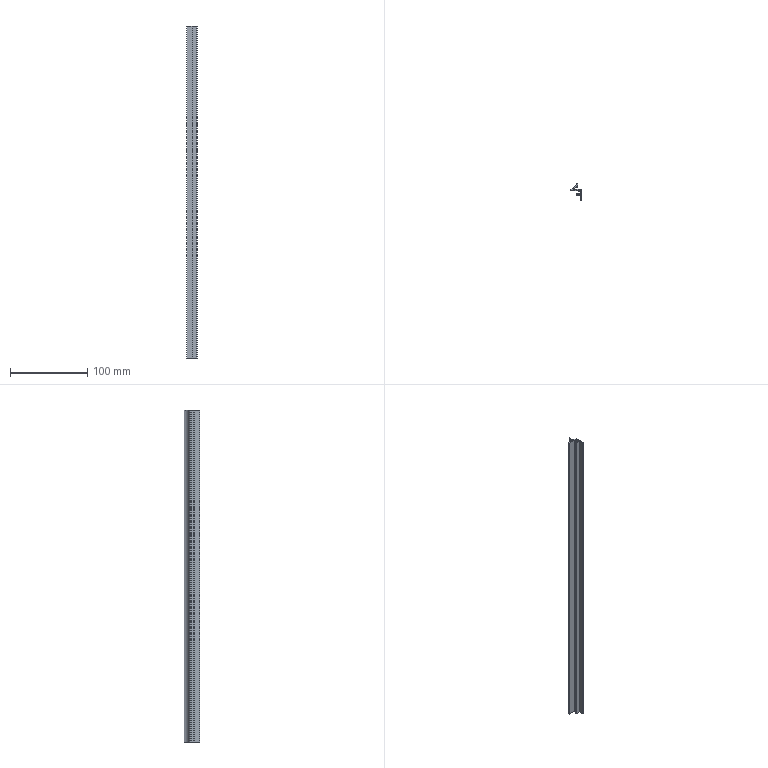Part | SolidWorks | features BaseBody 1, ICE 1, MoveFace 1 | 1 solid | 27 faces | box 14 x 20.3 x 430 mm | volume 21894 mm3 | plane 20 | cylinder 7 | commonest cylinder face diameters 0.387 x2 0.8 x2 0.4 x1 20 x1 22 x1
STEP:
#1=CARTESIAN_POINT('',(-5.304,-0.625,200.));
#2=VERTEX_POINT('',#1);
#3=CARTESIAN_POINT('',(-5.449,-0.8125,200.));
#4=VERTEX_POINT('',#3);
#5=CARTESIAN_POINT('',(-5.255,-0.8125,200.));
#6=DIRECTION('',(0.,0.,1.));
#7=DIRECTION('',(-1.,0.,0.));
#8=AXIS2_PLACEMENT_3D('',#5,#6,#7);
#9=CIRCLE('',#8,0.1937);
#10=EDGE_CURVE('',#2,#4,#9,.T.);
#11=ORIENTED_EDGE('',*,*,#10,.T.);
#12=CARTESIAN_POINT('',(-5.449,-0.8125,-230.));
#13=VERTEX_POINT('',#12);
#14=CARTESIAN_POINT('',(-5.449,-0.8125,230.));
#15=DIRECTION('',(0.,0.,-1.));
#16=VECTOR('',#15,1000.);
#17=LINE('',#14,#16);
#18=EDGE_CURVE('',#4,#13,#17,.T.);
#19=ORIENTED_EDGE('',*,*,#18,.T.);
#20=CARTESIAN_POINT('',(-5.304,-0.625,-230.));
#21=VERTEX_POINT('',#20);
#22=CARTESIAN_POINT('',(-5.255,-0.8125,-230.));
#23=DIRECTION('',(0.,0.,-1.));
#24=DIRECTION('',(1.,0.,0.));
#25=AXIS2_PLACEMENT_3D('',#22,#23,#24);
#26=CIRCLE('',#25,0.1937);
#27=EDGE_CURVE('',#13,#21,#26,.T.);
#28=ORIENTED_EDGE('',*,*,#27,.T.);
#29=CARTESIAN_POINT('',(-5.304,-0.625,230.));
#30=DIRECTION('',(0.,0.,-1.));
#31=VECTOR('',#30,1000.);
#32=LINE('',#29,#31);
#33=EDGE_CURVE('',#2,#21,#32,.T.);
#34=ORIENTED_EDGE('',*,*,#33,.F.);
#35=EDGE_LOOP('',(#11,#19,#28,#34));
#36=FACE_OUTER_BOUND('',#35,.T.);
#37=CARTESIAN_POINT('',(-5.255,-0.8125,230.));
#38=DIRECTION('',(0.,0.,-1.));
#39=DIRECTION('',(-1.,0.,0.));
#40=AXIS2_PLACEMENT_3D('',#37,#38,#39);
#41=CYLINDRICAL_SURFACE('',#40,0.1937);
#42=ADVANCED_FACE('',(#36),#41,.F.);
#43=CARTESIAN_POINT('',(5.,-1.,-230.));
#44=VERTEX_POINT('',#43);
#45=CARTESIAN_POINT('',(5.,-14.3,-230.));
#46=VERTEX_POINT('',#45);
#47=CARTESIAN_POINT('',(5.,29.623,-230.));
#48=DIRECTION('',(0.,-1.,0.));
#49=VECTOR('',#48,1000.);
#50=LINE('',#47,#49);
#51=EDGE_CURVE('',#44,#46,#50,.T.);
#52=ORIENTED_EDGE('',*,*,#51,.F.);
#53=CARTESIAN_POINT('',(5.,-1.,200.));
#54=VERTEX_POINT('',#53);
#55=CARTESIAN_POINT('',(5.,-1.,230.));
#56=DIRECTION('',(0.,0.,-1.));
#57=VECTOR('',#56,1000.);
#58=LINE('',#55,#57);
#59=EDGE_CURVE('',#54,#44,#58,.T.);
#60=ORIENTED_EDGE('',*,*,#59,.F.);
#61=CARTESIAN_POINT('',(5.,-14.3,200.));
#62=VERTEX_POINT('',#61);
#63=CARTESIAN_POINT('',(5.,-14.3,200.));
#64=DIRECTION('',(0.,1.,0.));
#65=VECTOR('',#64,1000.);
#66=LINE('',#63,#65);
#67=EDGE_CURVE('',#62,#54,#66,.T.);
#68=ORIENTED_EDGE('',*,*,#67,.F.);
#69=CARTESIAN_POINT('',(5.,-14.3,230.));
#70=DIRECTION('',(0.,0.,1.));
#71=VECTOR('',#70,1000.);
#72=LINE('',#69,#71);
#73=EDGE_CURVE('',#46,#62,#72,.T.);
#74=ORIENTED_EDGE('',*,*,#73,.F.);
#75=EDGE_LOOP('',(#52,#60,#68,#74));
#76=FACE_OUTER_BOUND('',#75,.T.);
#77=CARTESIAN_POINT('',(5.,-14.3,230.));
#78=DIRECTION('',(-1.,0.,0.));
#79=DIRECTION('',(0.,0.,1.));
#80=AXIS2_PLACEMENT_3D('',#77,#78,#79);
#81=PLANE('',#80);
#82=ADVANCED_FACE('',(#76),#81,.F.);
#83=CARTESIAN_POINT('',(-9.,-2.,-230.));
#84=VERTEX_POINT('',#83);
#85=CARTESIAN_POINT('',(-9.,-2.,200.));
#86=VERTEX_POINT('',#85);
#87=CARTESIAN_POINT('',(-9.,-2.,230.));
#88=DIRECTION('',(0.,0.,1.));
#89=VECTOR('',#88,1000.);
#90=LINE('',#87,#89);
#91=EDGE_CURVE('',#84,#86,#90,.T.);
#92=ORIENTED_EDGE('',*,*,#91,.F.);
#93=CARTESIAN_POINT('',(0.9,-2.,-230.));
#94=VERTEX_POINT('',#93);
#95=CARTESIAN_POINT('',(5.,-2.,-230.));
#96=DIRECTION('',(-1.,0.,0.));
#97=VECTOR('',#96,1000.);
#98=LINE('',#95,#97);
#99=EDGE_CURVE('',#94,#84,#98,.T.);
#100=ORIENTED_EDGE('',*,*,#99,.F.);
#101=CARTESIAN_POINT('',(0.9,-2.,200.));
#102=VERTEX_POINT('',#101);
#103=CARTESIAN_POINT('',(0.9,-2.,230.));
#104=DIRECTION('',(0.,0.,-1.));
#105=VECTOR('',#104,1000.);
#106=LINE('',#103,#105);
#107=EDGE_CURVE('',#102,#94,#106,.T.);
#108=ORIENTED_EDGE('',*,*,#107,.F.);
#109=CARTESIAN_POINT('',(5.,-2.,200.));
#110=DIRECTION('',(1.,0.,0.));
#111=VECTOR('',#110,1000.);
#112=LINE('',#109,#111);
#113=EDGE_CURVE('',#86,#102,#112,.T.);
#114=ORIENTED_EDGE('',*,*,#113,.F.);
#115=EDGE_LOOP('',(#92,#100,#108,#114));
#116=FACE_OUTER_BOUND('',#115,.T.);
#117=CARTESIAN_POINT('',(-9.,-2.,230.));
#118=DIRECTION('',(0.,1.,0.));
#119=DIRECTION('',(0.,0.,1.));
#120=AXIS2_PLACEMENT_3D('',#117,#118,#119);
#121=PLANE('',#120);
#122=ADVANCED_FACE('',(#116),#121,.F.);
#123=CARTESIAN_POINT('',(4.,-6.,200.));
#124=VERTEX_POINT('',#123);
#125=CARTESIAN_POINT('',(4.,-3.,200.));
#126=VERTEX_POINT('',#125);
#127=CARTESIAN_POINT('',(4.,29.623,200.));
#128=DIRECTION('',(0.,1.,0.));
#129=VECTOR('',#128,1000.);
#130=LINE('',#127,#129);
#131=EDGE_CURVE('',#124,#126,#130,.T.);
#132=ORIENTED_EDGE('',*,*,#131,.F.);
#133=CARTESIAN_POINT('',(1.,-6.,200.));
#134=VERTEX_POINT('',#133);
#135=CARTESIAN_POINT('',(5.,-6.,200.));
#136=DIRECTION('',(1.,0.,0.));
#137=VECTOR('',#136,1000.);
#138=LINE('',#135,#137);
#139=EDGE_CURVE('',#134,#124,#138,.T.);
#140=ORIENTED_EDGE('',*,*,#139,.F.);
#141=CARTESIAN_POINT('',(1.,-6.7,200.));
#142=VERTEX_POINT('',#141);
#143=CARTESIAN_POINT('',(1.,-6.,200.));
#144=DIRECTION('',(0.,-1.,0.));
#145=VECTOR('',#144,1000.);
#146=LINE('',#143,#145);
#147=EDGE_CURVE('',#134,#142,#146,.T.);
#148=ORIENTED_EDGE('',*,*,#147,.T.);
#149=CARTESIAN_POINT('',(-1.7,-6.7,200.));
#150=VERTEX_POINT('',#149);
#151=CARTESIAN_POINT('',(5.,-6.7,200.));
#152=DIRECTION('',(1.,0.,0.));
#153=VECTOR('',#152,1000.);
#154=LINE('',#151,#153);
#155=EDGE_CURVE('',#150,#142,#154,.T.);
#156=ORIENTED_EDGE('',*,*,#155,.F.);
#157=CARTESIAN_POINT('',(-1.7,-7.7,200.));
#158=VERTEX_POINT('',#157);
#159=CARTESIAN_POINT('',(-1.7,-6.7,200.));
#160=DIRECTION('',(0.,-1.,0.));
#161=VECTOR('',#160,1000.);
#162=LINE('',#159,#161);
#163=EDGE_CURVE('',#150,#158,#162,.T.);
#164=ORIENTED_EDGE('',*,*,#163,.T.);
#165=CARTESIAN_POINT('',(4.,-7.7,200.));
#166=VERTEX_POINT('',#165);
#167=CARTESIAN_POINT('',(5.,-7.7,200.));
#168=DIRECTION('',(-1.,0.,0.));
#169=VECTOR('',#168,1000.);
#170=LINE('',#167,#169);
#171=EDGE_CURVE('',#166,#158,#170,.T.);
#172=ORIENTED_EDGE('',*,*,#171,.F.);
#173=CARTESIAN_POINT('',(4.,-14.3,200.));
#174=VERTEX_POINT('',#173);
#175=CARTESIAN_POINT('',(4.,29.623,200.));
#176=DIRECTION('',(0.,1.,0.));
#177=VECTOR('',#176,1000.);
#178=LINE('',#175,#177);
#179=EDGE_CURVE('',#174,#166,#178,.T.);
#180=ORIENTED_EDGE('',*,*,#179,.F.);
#181=CARTESIAN_POINT('',(5.,-14.3,200.));
#182=DIRECTION('',(-1.,0.,0.));
#183=VECTOR('',#182,1000.);
#184=LINE('',#181,#183);
#185=EDGE_CURVE('',#62,#174,#184,.T.);
#186=ORIENTED_EDGE('',*,*,#185,.F.);
#187=ORIENTED_EDGE('',*,*,#67,.T.);
#188=CARTESIAN_POINT('',(-5.207,-1.,200.));
#189=VERTEX_POINT('',#188);
#190=CARTESIAN_POINT('',(5.,-1.,200.));
#191=DIRECTION('',(1.,0.,0.));
#192=VECTOR('',#191,1000.);
#193=LINE('',#190,#192);
#194=EDGE_CURVE('',#189,#54,#193,.T.);
#195=ORIENTED_EDGE('',*,*,#194,.F.);
#196=CARTESIAN_POINT('',(-5.255,-0.8125,200.));
#197=DIRECTION('',(0.,0.,1.));
#198=DIRECTION('',(-1.,0.,0.));
#199=AXIS2_PLACEMENT_3D('',#196,#197,#198);
#200=CIRCLE('',#199,0.1937);
#201=EDGE_CURVE('',#4,#189,#200,.T.);
#202=ORIENTED_EDGE('',*,*,#201,.F.);
#203=ORIENTED_EDGE('',*,*,#10,.F.);
#204=CARTESIAN_POINT('',(-1.368,3.063,200.));
#205=VERTEX_POINT('',#204);
#206=CARTESIAN_POINT('',(-10.628,9.,200.));
#207=DIRECTION('',(0.,0.,1.));
#208=DIRECTION('',(-1.,0.,0.));
#209=AXIS2_PLACEMENT_3D('',#206,#207,#208);
#210=CIRCLE('',#209,11.);
#211=EDGE_CURVE('',#2,#205,#210,.T.);
#212=ORIENTED_EDGE('',*,*,#211,.T.);
#213=CARTESIAN_POINT('',(-1.,2.955,200.));
#214=VERTEX_POINT('',#213);
#215=CARTESIAN_POINT('',(-1.2,2.955,200.));
#216=DIRECTION('',(0.,0.,1.));
#217=DIRECTION('',(-1.,0.,0.));
#218=AXIS2_PLACEMENT_3D('',#215,#216,#217);
#219=CIRCLE('',#218,0.2);
#220=EDGE_CURVE('',#214,#205,#219,.T.);
#221=ORIENTED_EDGE('',*,*,#220,.F.);
#222=CARTESIAN_POINT('',(-1.,1.5,200.));
#223=VERTEX_POINT('',#222);
#224=CARTESIAN_POINT('',(-1.,2.955,200.));
#225=DIRECTION('',(0.,1.,0.));
#226=VECTOR('',#225,1000.);
#227=LINE('',#224,#226);
#228=EDGE_CURVE('',#223,#214,#227,.T.);
#229=ORIENTED_EDGE('',*,*,#228,.F.);
#230=CARTESIAN_POINT('',(0.,1.5,200.));
#231=VERTEX_POINT('',#230);
#232=CARTESIAN_POINT('',(-1.,1.5,200.));
#233=DIRECTION('',(-1.,0.,0.));
#234=VECTOR('',#233,1000.);
#235=LINE('',#232,#234);
#236=EDGE_CURVE('',#231,#223,#235,.T.);
#237=ORIENTED_EDGE('',*,*,#236,.F.);
#238=CARTESIAN_POINT('',(0.,6.,200.));
#239=VERTEX_POINT('',#238);
#240=CARTESIAN_POINT('',(0.,1.5,200.));
#241=DIRECTION('',(0.,-1.,0.));
#242=VECTOR('',#241,1000.);
#243=LINE('',#240,#242);
#244=EDGE_CURVE('',#239,#231,#243,.T.);
#245=ORIENTED_EDGE('',*,*,#244,.F.);
#246=CARTESIAN_POINT('',(-0.8,6.,200.));
#247=VERTEX_POINT('',#246);
#248=CARTESIAN_POINT('',(0.,6.,200.));
#249=DIRECTION('',(1.,0.,0.));
#250=VECTOR('',#249,1000.);
#251=LINE('',#248,#250);
#252=EDGE_CURVE('',#247,#239,#251,.T.);
#253=ORIENTED_EDGE('',*,*,#252,.F.);
#254=CARTESIAN_POINT('',(-1.178,5.731,200.));
#255=VERTEX_POINT('',#254);
#256=CARTESIAN_POINT('',(-0.8,5.6,200.));
#257=DIRECTION('',(0.,0.,1.));
#258=DIRECTION('',(-1.,0.,0.));
#259=AXIS2_PLACEMENT_3D('',#256,#257,#258);
#260=CIRCLE('',#259,0.4);
#261=EDGE_CURVE('',#247,#255,#260,.T.);
#262=ORIENTED_EDGE('',*,*,#261,.T.);
#263=CARTESIAN_POINT('',(-8.678,-0.8077,200.));
#264=VERTEX_POINT('',#263);
#265=CARTESIAN_POINT('',(-10.628,9.,200.));
#266=DIRECTION('',(0.,0.,1.));
#267=DIRECTION('',(-1.,0.,0.));
#268=AXIS2_PLACEMENT_3D('',#265,#266,#267);
#269=CIRCLE('',#268,10.);
#270=EDGE_CURVE('',#264,#255,#269,.T.);
#271=ORIENTED_EDGE('',*,*,#270,.F.);
#272=CARTESIAN_POINT('',(-9.,-1.2,200.));
#273=VERTEX_POINT('',#272);
#274=CARTESIAN_POINT('',(-8.6,-1.2,200.));
#275=DIRECTION('',(0.,0.,1.));
#276=DIRECTION('',(-1.,0.,0.));
#277=AXIS2_PLACEMENT_3D('',#274,#275,#276);
#278=CIRCLE('',#277,0.4);
#279=EDGE_CURVE('',#264,#273,#278,.T.);
#280=ORIENTED_EDGE('',*,*,#279,.T.);
#281=CARTESIAN_POINT('',(-9.,8.,200.));
#282=DIRECTION('',(0.,-1.,0.));
#283=VECTOR('',#282,1000.);
#284=LINE('',#281,#283);
#285=EDGE_CURVE('',#273,#86,#284,.T.);
#286=ORIENTED_EDGE('',*,*,#285,.T.);
#287=ORIENTED_EDGE('',*,*,#113,.T.);
#288=CARTESIAN_POINT('',(0.9,-3.,200.));
#289=VERTEX_POINT('',#288);
#290=CARTESIAN_POINT('',(0.9,29.623,200.));
#291=DIRECTION('',(0.,1.,0.));
#292=VECTOR('',#291,1000.);
#293=LINE('',#290,#292);
#294=EDGE_CURVE('',#289,#102,#293,.T.);
#295=ORIENTED_EDGE('',*,*,#294,.F.);
#296=CARTESIAN_POINT('',(5.,-3.,200.));
#297=DIRECTION('',(-1.,0.,0.));
#298=VECTOR('',#297,1000.);
#299=LINE('',#296,#298);
#300=EDGE_CURVE('',#126,#289,#299,.T.);
#301=ORIENTED_EDGE('',*,*,#300,.F.);
#302=EDGE_LOOP('',(#132,#140,#148,#156,#164,#172,#180,#186,#187,#195,#202,#203,#212,#221,#229,#237,#245,#253,#262,#271,#280,#286,#287,#295,#301));
#303=FACE_OUTER_BOUND('',#302,.T.);
#304=CARTESIAN_POINT('',(5.,29.623,200.));
#305=DIRECTION('',(0.,0.,-1.));
#306=DIRECTION('',(-1.,0.,0.));
#307=AXIS2_PLACEMENT_3D('',#304,#305,#306);
#308=PLANE('',#307);
#309=ADVANCED_FACE('',(#303),#308,.F.);
#310=ORIENTED_EDGE('',*,*,#185,.T.);
#311=CARTESIAN_POINT('',(4.,-14.3,-230.));
#312=VERTEX_POINT('',#311);
#313=CARTESIAN_POINT('',(4.,-14.3,230.));
#314=DIRECTION('',(0.,0.,1.));
#315=VECTOR('',#314,1000.);
#316=LINE('',#313,#315);
#317=EDGE_CURVE('',#312,#174,#316,.T.);
#318=ORIENTED_EDGE('',*,*,#317,.F.);
#319=CARTESIAN_POINT('',(5.,-14.3,-230.));
#320=DIRECTION('',(-1.,0.,0.));
#321=VECTOR('',#320,1000.);
#322=LINE('',#319,#321);
#323=EDGE_CURVE('',#46,#312,#322,.T.);
#324=ORIENTED_EDGE('',*,*,#323,.F.);
#325=ORIENTED_EDGE('',*,*,#73,.T.);
#326=EDGE_LOOP('',(#310,#318,#324,#325));
#327=FACE_OUTER_BOUND('',#326,.T.);
#328=CARTESIAN_POINT('',(4.,-14.3,230.));
#329=DIRECTION('',(0.,1.,0.));
#330=DIRECTION('',(0.,0.,1.));
#331=AXIS2_PLACEMENT_3D('',#328,#329,#330);
#332=PLANE('',#331);
#333=ADVANCED_FACE('',(#327),#332,.F.);
#334=ORIENTED_EDGE('',*,*,#51,.T.);
#335=ORIENTED_EDGE('',*,*,#323,.T.);
#336=CARTESIAN_POINT('',(4.,-7.7,-230.));
#337=VERTEX_POINT('',#336);
#338=CARTESIAN_POINT('',(4.,-7.7,-230.));
#339=DIRECTION('',(0.,-1.,0.));
#340=VECTOR('',#339,1000.);
#341=LINE('',#338,#340);
#342=EDGE_CURVE('',#337,#312,#341,.T.);
#343=ORIENTED_EDGE('',*,*,#342,.F.);
#344=CARTESIAN_POINT('',(-1.7,-7.7,-230.));
#345=VERTEX_POINT('',#344);
#346=CARTESIAN_POINT('',(-1.7,-7.7,-230.));
#347=DIRECTION('',(1.,0.,0.));
#348=VECTOR('',#347,1000.);
#349=LINE('',#346,#348);
#350=EDGE_CURVE('',#345,#337,#349,.T.);
#351=ORIENTED_EDGE('',*,*,#350,.F.);
#352=CARTESIAN_POINT('',(-1.7,-6.7,-230.));
#353=VERTEX_POINT('',#352);
#354=CARTESIAN_POINT('',(-1.7,29.623,-230.));
#355=DIRECTION('',(0.,1.,0.));
#356=VECTOR('',#355,1000.);
#357=LINE('',#354,#356);
#358=EDGE_CURVE('',#345,#353,#357,.T.);
#359=ORIENTED_EDGE('',*,*,#358,.T.);
#360=CARTESIAN_POINT('',(1.,-6.7,-230.));
#361=VERTEX_POINT('',#360);
#362=CARTESIAN_POINT('',(1.,-6.7,-230.));
#363=DIRECTION('',(-1.,0.,0.));
#364=VECTOR('',#363,1000.);
#365=LINE('',#362,#364);
#366=EDGE_CURVE('',#361,#353,#365,.T.);
#367=ORIENTED_EDGE('',*,*,#366,.F.);
#368=CARTESIAN_POINT('',(1.,-6.,-230.));
#369=VERTEX_POINT('',#368);
#370=CARTESIAN_POINT('',(1.,29.623,-230.));
#371=DIRECTION('',(0.,1.,0.));
#372=VECTOR('',#371,1000.);
#373=LINE('',#370,#372);
#374=EDGE_CURVE('',#361,#369,#373,.T.);
#375=ORIENTED_EDGE('',*,*,#374,.T.);
#376=CARTESIAN_POINT('',(4.,-6.,-230.));
#377=VERTEX_POINT('',#376);
#378=CARTESIAN_POINT('',(4.,-6.,-230.));
#379=DIRECTION('',(-1.,0.,0.));
#380=VECTOR('',#379,1000.);
#381=LINE('',#378,#380);
#382=EDGE_CURVE('',#377,#369,#381,.T.);
#383=ORIENTED_EDGE('',*,*,#382,.F.);
#384=CARTESIAN_POINT('',(4.,-3.,-230.));
#385=VERTEX_POINT('',#384);
#386=CARTESIAN_POINT('',(4.,-3.,-230.));
#387=DIRECTION('',(0.,-1.,0.));
#388=VECTOR('',#387,1000.);
#389=LINE('',#386,#388);
#390=EDGE_CURVE('',#385,#377,#389,.T.);
#391=ORIENTED_EDGE('',*,*,#390,.F.);
#392=CARTESIAN_POINT('',(0.9,-3.,-230.));
#393=VERTEX_POINT('',#392);
#394=CARTESIAN_POINT('',(0.9,-3.,-230.));
#395=DIRECTION('',(1.,0.,0.));
#396=VECTOR('',#395,1000.);
#397=LINE('',#394,#396);
#398=EDGE_CURVE('',#393,#385,#397,.T.);
#399=ORIENTED_EDGE('',*,*,#398,.F.);
#400=CARTESIAN_POINT('',(0.9,-2.,-230.));
#401=DIRECTION('',(0.,-1.,0.));
#402=VECTOR('',#401,1000.);
#403=LINE('',#400,#402);
#404=EDGE_CURVE('',#94,#393,#403,.T.);
#405=ORIENTED_EDGE('',*,*,#404,.F.);
#406=ORIENTED_EDGE('',*,*,#99,.T.);
#407=CARTESIAN_POINT('',(-9.,-1.2,-230.));
#408=VERTEX_POINT('',#407);
#409=CARTESIAN_POINT('',(-9.,-1.2,-230.));
#410=DIRECTION('',(0.,-1.,0.));
#411=VECTOR('',#410,1000.);
#412=LINE('',#409,#411);
#413=EDGE_CURVE('',#408,#84,#412,.T.);
#414=ORIENTED_EDGE('',*,*,#413,.F.);
#415=CARTESIAN_POINT('',(-8.678,-0.8077,-230.));
#416=VERTEX_POINT('',#415);
#417=CARTESIAN_POINT('',(-8.6,-1.2,-230.));
#418=DIRECTION('',(0.,0.,-1.));
#419=DIRECTION('',(1.,0.,0.));
#420=AXIS2_PLACEMENT_3D('',#417,#418,#419);
#421=CIRCLE('',#420,0.4);
#422=EDGE_CURVE('',#408,#416,#421,.T.);
#423=ORIENTED_EDGE('',*,*,#422,.T.);
#424=CARTESIAN_POINT('',(-1.178,5.731,-230.));
#425=VERTEX_POINT('',#424);
#426=CARTESIAN_POINT('',(-10.628,9.,-230.));
#427=DIRECTION('',(0.,0.,-1.));
#428=DIRECTION('',(1.,0.,0.));
#429=AXIS2_PLACEMENT_3D('',#426,#427,#428);
#430=CIRCLE('',#429,10.);
#431=EDGE_CURVE('',#425,#416,#430,.T.);
#432=ORIENTED_EDGE('',*,*,#431,.F.);
#433=CARTESIAN_POINT('',(-0.8,6.,-230.));
#434=VERTEX_POINT('',#433);
#435=CARTESIAN_POINT('',(-0.8,5.6,-230.));
#436=DIRECTION('',(0.,0.,-1.));
#437=DIRECTION('',(1.,0.,0.));
#438=AXIS2_PLACEMENT_3D('',#435,#436,#437);
#439=CIRCLE('',#438,0.4);
#440=EDGE_CURVE('',#425,#434,#439,.T.);
#441=ORIENTED_EDGE('',*,*,#440,.T.);
#442=CARTESIAN_POINT('',(0.,6.,-230.));
#443=VERTEX_POINT('',#442);
#444=CARTESIAN_POINT('',(0.,6.,-230.));
#445=DIRECTION('',(-1.,0.,0.));
#446=VECTOR('',#445,1000.);
#447=LINE('',#444,#446);
#448=EDGE_CURVE('',#443,#434,#447,.T.);
#449=ORIENTED_EDGE('',*,*,#448,.F.);
#450=CARTESIAN_POINT('',(0.,1.5,-230.));
#451=VERTEX_POINT('',#450);
#452=CARTESIAN_POINT('',(0.,1.5,-230.));
#453=DIRECTION('',(0.,1.,0.));
#454=VECTOR('',#453,1000.);
#455=LINE('',#452,#454);
#456=EDGE_CURVE('',#451,#443,#455,.T.);
#457=ORIENTED_EDGE('',*,*,#456,.F.);
#458=CARTESIAN_POINT('',(-1.,1.5,-230.));
#459=VERTEX_POINT('',#458);
#460=CARTESIAN_POINT('',(-1.,1.5,-230.));
#461=DIRECTION('',(1.,0.,0.));
#462=VECTOR('',#461,1000.);
#463=LINE('',#460,#462);
#464=EDGE_CURVE('',#459,#451,#463,.T.);
#465=ORIENTED_EDGE('',*,*,#464,.F.);
#466=CARTESIAN_POINT('',(-1.,2.955,-230.));
#467=VERTEX_POINT('',#466);
#468=CARTESIAN_POINT('',(-1.,2.955,-230.));
#469=DIRECTION('',(0.,-1.,0.));
#470=VECTOR('',#469,1000.);
#471=LINE('',#468,#470);
#472=EDGE_CURVE('',#467,#459,#471,.T.);
#473=ORIENTED_EDGE('',*,*,#472,.F.);
#474=CARTESIAN_POINT('',(-1.368,3.063,-230.));
#475=VERTEX_POINT('',#474);
#476=CARTESIAN_POINT('',(-1.2,2.955,-230.));
#477=DIRECTION('',(0.,0.,-1.));
#478=DIRECTION('',(1.,0.,0.));
#479=AXIS2_PLACEMENT_3D('',#476,#477,#478);
#480=CIRCLE('',#479,0.2);
#481=EDGE_CURVE('',#475,#467,#480,.T.);
#482=ORIENTED_EDGE('',*,*,#481,.F.);
#483=CARTESIAN_POINT('',(-10.628,9.,-230.));
#484=DIRECTION('',(0.,0.,-1.));
#485=DIRECTION('',(1.,0.,0.));
#486=AXIS2_PLACEMENT_3D('',#483,#484,#485);
#487=CIRCLE('',#486,11.);
#488=EDGE_CURVE('',#475,#21,#487,.T.);
#489=ORIENTED_EDGE('',*,*,#488,.T.);
#490=ORIENTED_EDGE('',*,*,#27,.F.);
#491=CARTESIAN_POINT('',(-5.207,-1.,-230.));
#492=VERTEX_POINT('',#491);
#493=CARTESIAN_POINT('',(-5.255,-0.8125,-230.));
#494=DIRECTION('',(0.,0.,-1.));
#495=DIRECTION('',(1.,0.,0.));
#496=AXIS2_PLACEMENT_3D('',#493,#494,#495);
#497=CIRCLE('',#496,0.1937);
#498=EDGE_CURVE('',#492,#13,#497,.T.);
#499=ORIENTED_EDGE('',*,*,#498,.F.);
#500=CARTESIAN_POINT('',(5.,-1.,-230.));
#501=DIRECTION('',(-1.,0.,0.));
#502=VECTOR('',#501,1000.);
#503=LINE('',#500,#502);
#504=EDGE_CURVE('',#44,#492,#503,.T.);
#505=ORIENTED_EDGE('',*,*,#504,.F.);
#506=EDGE_LOOP('',(#334,#335,#343,#351,#359,#367,#375,#383,#391,#399,#405,#406,#414,#423,#432,#441,#449,#457,#465,#473,#482,#489,#490,#499,#505));
#507=FACE_OUTER_BOUND('',#506,.T.);
#508=CARTESIAN_POINT('',(5.,29.623,-230.));
#509=DIRECTION('',(0.,0.,1.));
#510=DIRECTION('',(1.,0.,0.));
#511=AXIS2_PLACEMENT_3D('',#508,#509,#510);
#512=PLANE('',#511);
#513=ADVANCED_FACE('',(#507),#512,.F.);
#514=ORIENTED_EDGE('',*,*,#59,.T.);
#515=ORIENTED_EDGE('',*,*,#504,.T.);
#516=CARTESIAN_POINT('',(-5.207,-1.,230.));
#517=DIRECTION('',(0.,0.,-1.));
#518=VECTOR('',#517,1000.);
#519=LINE('',#516,#518);
#520=EDGE_CURVE('',#189,#492,#519,.T.);
#521=ORIENTED_EDGE('',*,*,#520,.F.);
#522=ORIENTED_EDGE('',*,*,#194,.T.);
#523=EDGE_LOOP('',(#514,#515,#521,#522));
#524=FACE_OUTER_BOUND('',#523,.T.);
#525=CARTESIAN_POINT('',(5.,-1.,230.));
#526=DIRECTION('',(0.,-1.,0.));
#527=DIRECTION('',(0.,0.,-1.));
#528=AXIS2_PLACEMENT_3D('',#525,#526,#527);
#529=PLANE('',#528);
#530=ADVANCED_FACE('',(#524),#529,.F.);
#531=CARTESIAN_POINT('',(-9.,-1.2,230.));
#532=DIRECTION('',(0.,0.,1.));
#533=VECTOR('',#532,1000.);
#534=LINE('',#531,#533);
#535=EDGE_CURVE('',#408,#273,#534,.T.);
#536=ORIENTED_EDGE('',*,*,#535,.F.);
#537=ORIENTED_EDGE('',*,*,#413,.T.);
#538=ORIENTED_EDGE('',*,*,#91,.T.);
#539=ORIENTED_EDGE('',*,*,#285,.F.);
#540=EDGE_LOOP('',(#536,#537,#538,#539));
#541=FACE_OUTER_BOUND('',#540,.T.);
#542=CARTESIAN_POINT('',(-9.,-1.2,230.));
#543=DIRECTION('',(1.,0.,0.));
#544=DIRECTION('',(0.,0.,-1.));
#545=AXIS2_PLACEMENT_3D('',#542,#543,#544);
#546=PLANE('',#545);
#547=ADVANCED_FACE('',(#541),#546,.F.);
#548=ORIENTED_EDGE('',*,*,#294,.T.);
#549=ORIENTED_EDGE('',*,*,#107,.T.);
#550=ORIENTED_EDGE('',*,*,#404,.T.);
#551=CARTESIAN_POINT('',(0.9,-3.,230.));
#552=DIRECTION('',(0.,0.,-1.));
#553=VECTOR('',#552,1000.);
#554=LINE('',#551,#553);
#555=EDGE_CURVE('',#289,#393,#554,.T.);
#556=ORIENTED_EDGE('',*,*,#555,.F.);
#557=EDGE_LOOP('',(#548,#549,#550,#556));
#558=FACE_OUTER_BOUND('',#557,.T.);
#559=CARTESIAN_POINT('',(0.9,-2.,230.));
#560=DIRECTION('',(1.,0.,0.));
#561=DIRECTION('',(0.,0.,-1.));
#562=AXIS2_PLACEMENT_3D('',#559,#560,#561);
#563=PLANE('',#562);
#564=ADVANCED_FACE('',(#558),#563,.F.);
#565=ORIENTED_EDGE('',*,*,#300,.T.);
#566=ORIENTED_EDGE('',*,*,#555,.T.);
#567=ORIENTED_EDGE('',*,*,#398,.T.);
#568=CARTESIAN_POINT('',(4.,-3.,230.));
#569=DIRECTION('',(0.,0.,-1.));
#570=VECTOR('',#569,1000.);
#571=LINE('',#568,#570);
#572=EDGE_CURVE('',#126,#385,#571,.T.);
#573=ORIENTED_EDGE('',*,*,#572,.F.);
#574=EDGE_LOOP('',(#565,#566,#567,#573));
#575=FACE_OUTER_BOUND('',#574,.T.);
#576=CARTESIAN_POINT('',(0.9,-3.,230.));
#577=DIRECTION('',(0.,1.,0.));
#578=DIRECTION('',(0.,0.,1.));
#579=AXIS2_PLACEMENT_3D('',#576,#577,#578);
#580=PLANE('',#579);
#581=ADVANCED_FACE('',(#575),#580,.F.);
#582=ORIENTED_EDGE('',*,*,#131,.T.);
#583=ORIENTED_EDGE('',*,*,#572,.T.);
#584=ORIENTED_EDGE('',*,*,#390,.T.);
#585=CARTESIAN_POINT('',(4.,-6.,230.));
#586=DIRECTION('',(0.,0.,-1.));
#587=VECTOR('',#586,1000.);
#588=LINE('',#585,#587);
#589=EDGE_CURVE('',#124,#377,#588,.T.);
#590=ORIENTED_EDGE('',*,*,#589,.F.);
#591=EDGE_LOOP('',(#582,#583,#584,#590));
#592=FACE_OUTER_BOUND('',#591,.T.);
#593=CARTESIAN_POINT('',(4.,-3.,230.));
#594=DIRECTION('',(1.,0.,0.));
#595=DIRECTION('',(0.,0.,-1.));
#596=AXIS2_PLACEMENT_3D('',#593,#594,#595);
#597=PLANE('',#596);
#598=ADVANCED_FACE('',(#592),#597,.F.);
#599=ORIENTED_EDGE('',*,*,#139,.T.);
#600=ORIENTED_EDGE('',*,*,#589,.T.);
#601=ORIENTED_EDGE('',*,*,#382,.T.);
#602=CARTESIAN_POINT('',(1.,-6.,230.));
#603=DIRECTION('',(0.,0.,-1.));
#604=VECTOR('',#603,1000.);
#605=LINE('',#602,#604);
#606=EDGE_CURVE('',#134,#369,#605,.T.);
#607=ORIENTED_EDGE('',*,*,#606,.F.);
#608=EDGE_LOOP('',(#599,#600,#601,#607));
#609=FACE_OUTER_BOUND('',#608,.T.);
#610=CARTESIAN_POINT('',(4.,-6.,230.));
#611=DIRECTION('',(0.,-1.,0.));
#612=DIRECTION('',(0.,0.,-1.));
#613=AXIS2_PLACEMENT_3D('',#610,#611,#612);
#614=PLANE('',#613);
#615=ADVANCED_FACE('',(#609),#614,.F.);
#616=ORIENTED_EDGE('',*,*,#155,.T.);
#617=CARTESIAN_POINT('',(1.,-6.7,230.));
#618=DIRECTION('',(0.,0.,1.));
#619=VECTOR('',#618,1000.);
#620=LINE('',#617,#619);
#621=EDGE_CURVE('',#361,#142,#620,.T.);
#622=ORIENTED_EDGE('',*,*,#621,.F.);
#623=ORIENTED_EDGE('',*,*,#366,.T.);
#624=CARTESIAN_POINT('',(-1.7,-6.7,230.));
#625=DIRECTION('',(0.,0.,-1.));
#626=VECTOR('',#625,1000.);
#627=LINE('',#624,#626);
#628=EDGE_CURVE('',#150,#353,#627,.T.);
#629=ORIENTED_EDGE('',*,*,#628,.F.);
#630=EDGE_LOOP('',(#616,#622,#623,#629));
#631=FACE_OUTER_BOUND('',#630,.T.);
#632=CARTESIAN_POINT('',(1.,-6.7,230.));
#633=DIRECTION('',(0.,-1.,0.));
#634=DIRECTION('',(0.,0.,-1.));
#635=AXIS2_PLACEMENT_3D('',#632,#633,#634);
#636=PLANE('',#635);
#637=ADVANCED_FACE('',(#631),#636,.F.);
#638=ORIENTED_EDGE('',*,*,#171,.T.);
#639=CARTESIAN_POINT('',(-1.7,-7.7,230.));
#640=DIRECTION('',(0.,0.,1.));
#641=VECTOR('',#640,1000.);
#642=LINE('',#639,#641);
#643=EDGE_CURVE('',#345,#158,#642,.T.);
#644=ORIENTED_EDGE('',*,*,#643,.F.);
#645=ORIENTED_EDGE('',*,*,#350,.T.);
#646=CARTESIAN_POINT('',(4.,-7.7,230.));
#647=DIRECTION('',(0.,0.,-1.));
#648=VECTOR('',#647,1000.);
#649=LINE('',#646,#648);
#650=EDGE_CURVE('',#166,#337,#649,.T.);
#651=ORIENTED_EDGE('',*,*,#650,.F.);
#652=EDGE_LOOP('',(#638,#644,#645,#651));
#653=FACE_OUTER_BOUND('',#652,.T.);
#654=CARTESIAN_POINT('',(-1.7,-7.7,230.));
#655=DIRECTION('',(0.,1.,0.));
#656=DIRECTION('',(0.,0.,1.));
#657=AXIS2_PLACEMENT_3D('',#654,#655,#656);
#658=PLANE('',#657);
#659=ADVANCED_FACE('',(#653),#658,.F.);
#660=ORIENTED_EDGE('',*,*,#179,.T.);
#661=ORIENTED_EDGE('',*,*,#650,.T.);
#662=ORIENTED_EDGE('',*,*,#342,.T.);
#663=ORIENTED_EDGE('',*,*,#317,.T.);
#664=EDGE_LOOP('',(#660,#661,#662,#663));
#665=FACE_OUTER_BOUND('',#664,.T.);
#666=CARTESIAN_POINT('',(4.,-7.7,230.));
#667=DIRECTION('',(1.,0.,0.));
#668=DIRECTION('',(0.,0.,-1.));
#669=AXIS2_PLACEMENT_3D('',#666,#667,#668);
#670=PLANE('',#669);
#671=ADVANCED_FACE('',(#665),#670,.F.);
#672=ORIENTED_EDGE('',*,*,#18,.F.);
#673=ORIENTED_EDGE('',*,*,#201,.T.);
#674=ORIENTED_EDGE('',*,*,#520,.T.);
#675=ORIENTED_EDGE('',*,*,#498,.T.);
#676=EDGE_LOOP('',(#672,#673,#674,#675));
#677=FACE_OUTER_BOUND('',#676,.T.);
#678=CARTESIAN_POINT('',(-5.255,-0.8125,230.));
#679=DIRECTION('',(0.,0.,-1.));
#680=DIRECTION('',(-1.,0.,0.));
#681=AXIS2_PLACEMENT_3D('',#678,#679,#680);
#682=CYLINDRICAL_SURFACE('',#681,0.1937);
#683=ADVANCED_FACE('',(#677),#682,.F.);
#684=CARTESIAN_POINT('',(-1.,2.955,230.));
#685=DIRECTION('',(0.,0.,1.));
#686=VECTOR('',#685,1000.);
#687=LINE('',#684,#686);
#688=EDGE_CURVE('',#467,#214,#687,.T.);
#689=ORIENTED_EDGE('',*,*,#688,.F.);
#690=ORIENTED_EDGE('',*,*,#472,.T.);
#691=CARTESIAN_POINT('',(-1.,1.5,230.));
#692=DIRECTION('',(0.,0.,-1.));
#693=VECTOR('',#692,1000.);
#694=LINE('',#691,#693);
#695=EDGE_CURVE('',#223,#459,#694,.T.);
#696=ORIENTED_EDGE('',*,*,#695,.F.);
#697=ORIENTED_EDGE('',*,*,#228,.T.);
#698=EDGE_LOOP('',(#689,#690,#696,#697));
#699=FACE_OUTER_BOUND('',#698,.T.);
#700=CARTESIAN_POINT('',(-1.,2.955,230.));
#701=DIRECTION('',(1.,0.,0.));
#702=DIRECTION('',(0.,0.,-1.));
#703=AXIS2_PLACEMENT_3D('',#700,#701,#702);
#704=PLANE('',#703);
#705=ADVANCED_FACE('',(#699),#704,.F.);
#706=ORIENTED_EDGE('',*,*,#488,.F.);
#707=CARTESIAN_POINT('',(-1.368,3.063,230.));
#708=DIRECTION('',(0.,0.,1.));
#709=VECTOR('',#708,1000.);
#710=LINE('',#707,#709);
#711=EDGE_CURVE('',#475,#205,#710,.T.);
#712=ORIENTED_EDGE('',*,*,#711,.T.);
#713=ORIENTED_EDGE('',*,*,#211,.F.);
#714=ORIENTED_EDGE('',*,*,#33,.T.);
#715=EDGE_LOOP('',(#706,#712,#713,#714));
#716=FACE_OUTER_BOUND('',#715,.T.);
#717=CARTESIAN_POINT('',(-10.628,9.,230.));
#718=DIRECTION('',(0.,0.,-1.));
#719=DIRECTION('',(-1.,0.,0.));
#720=AXIS2_PLACEMENT_3D('',#717,#718,#719);
#721=CYLINDRICAL_SURFACE('',#720,11.);
#722=ADVANCED_FACE('',(#716),#721,.T.);
#723=CARTESIAN_POINT('',(-1.178,5.731,230.));
#724=DIRECTION('',(0.,0.,1.));
#725=VECTOR('',#724,1000.);
#726=LINE('',#723,#725);
#727=EDGE_CURVE('',#425,#255,#726,.T.);
#728=ORIENTED_EDGE('',*,*,#727,.F.);
#729=ORIENTED_EDGE('',*,*,#431,.T.);
#730=CARTESIAN_POINT('',(-8.678,-0.8077,230.));
#731=DIRECTION('',(0.,0.,-1.));
#732=VECTOR('',#731,1000.);
#733=LINE('',#730,#732);
#734=EDGE_CURVE('',#264,#416,#733,.T.);
#735=ORIENTED_EDGE('',*,*,#734,.F.);
#736=ORIENTED_EDGE('',*,*,#270,.T.);
#737=EDGE_LOOP('',(#728,#729,#735,#736));
#738=FACE_OUTER_BOUND('',#737,.T.);
#739=CARTESIAN_POINT('',(-10.628,9.,230.));
#740=DIRECTION('',(0.,0.,-1.));
#741=DIRECTION('',(-1.,0.,0.));
#742=AXIS2_PLACEMENT_3D('',#739,#740,#741);
#743=CYLINDRICAL_SURFACE('',#742,10.);
#744=ADVANCED_FACE('',(#738),#743,.F.);
#745=CARTESIAN_POINT('',(0.,1.5,230.));
#746=DIRECTION('',(0.,0.,1.));
#747=VECTOR('',#746,1000.);
#748=LINE('',#745,#747);
#749=EDGE_CURVE('',#451,#231,#748,.T.);
#750=ORIENTED_EDGE('',*,*,#749,.F.);
#751=ORIENTED_EDGE('',*,*,#456,.T.);
#752=CARTESIAN_POINT('',(0.,6.,230.));
#753=DIRECTION('',(0.,0.,-1.));
#754=VECTOR('',#753,1000.);
#755=LINE('',#752,#754);
#756=EDGE_CURVE('',#239,#443,#755,.T.);
#757=ORIENTED_EDGE('',*,*,#756,.F.);
#758=ORIENTED_EDGE('',*,*,#244,.T.);
#759=EDGE_LOOP('',(#750,#751,#757,#758));
#760=FACE_OUTER_BOUND('',#759,.T.);
#761=CARTESIAN_POINT('',(0.,1.5,230.));
#762=DIRECTION('',(-1.,0.,0.));
#763=DIRECTION('',(0.,0.,1.));
#764=AXIS2_PLACEMENT_3D('',#761,#762,#763);
#765=PLANE('',#764);
#766=ADVANCED_FACE('',(#760),#765,.F.);
#767=ORIENTED_EDGE('',*,*,#422,.F.);
#768=ORIENTED_EDGE('',*,*,#535,.T.);
#769=ORIENTED_EDGE('',*,*,#279,.F.);
#770=ORIENTED_EDGE('',*,*,#734,.T.);
#771=EDGE_LOOP('',(#767,#768,#769,#770));
#772=FACE_OUTER_BOUND('',#771,.T.);
#773=CARTESIAN_POINT('',(-8.6,-1.2,230.));
#774=DIRECTION('',(0.,0.,-1.));
#775=DIRECTION('',(-1.,0.,0.));
#776=AXIS2_PLACEMENT_3D('',#773,#774,#775);
#777=CYLINDRICAL_SURFACE('',#776,0.4);
#778=ADVANCED_FACE('',(#772),#777,.T.);
#779=ORIENTED_EDGE('',*,*,#147,.F.);
#780=ORIENTED_EDGE('',*,*,#606,.T.);
#781=ORIENTED_EDGE('',*,*,#374,.F.);
#782=ORIENTED_EDGE('',*,*,#621,.T.);
#783=EDGE_LOOP('',(#779,#780,#781,#782));
#784=FACE_OUTER_BOUND('',#783,.T.);
#785=CARTESIAN_POINT('',(1.,-6.,230.));
#786=DIRECTION('',(1.,0.,0.));
#787=DIRECTION('',(0.,0.,-1.));
#788=AXIS2_PLACEMENT_3D('',#785,#786,#787);
#789=PLANE('',#788);
#790=ADVANCED_FACE('',(#784),#789,.F.);
#791=ORIENTED_EDGE('',*,*,#163,.F.);
#792=ORIENTED_EDGE('',*,*,#628,.T.);
#793=ORIENTED_EDGE('',*,*,#358,.F.);
#794=ORIENTED_EDGE('',*,*,#643,.T.);
#795=EDGE_LOOP('',(#791,#792,#793,#794));
#796=FACE_OUTER_BOUND('',#795,.T.);
#797=CARTESIAN_POINT('',(-1.7,-6.7,230.));
#798=DIRECTION('',(1.,0.,0.));
#799=DIRECTION('',(0.,0.,-1.));
#800=AXIS2_PLACEMENT_3D('',#797,#798,#799);
#801=PLANE('',#800);
#802=ADVANCED_FACE('',(#796),#801,.F.);
#803=ORIENTED_EDGE('',*,*,#711,.F.);
#804=ORIENTED_EDGE('',*,*,#481,.T.);
#805=ORIENTED_EDGE('',*,*,#688,.T.);
#806=ORIENTED_EDGE('',*,*,#220,.T.);
#807=EDGE_LOOP('',(#803,#804,#805,#806));
#808=FACE_OUTER_BOUND('',#807,.T.);
#809=CARTESIAN_POINT('',(-1.2,2.955,230.));
#810=DIRECTION('',(0.,0.,-1.));
#811=DIRECTION('',(-1.,0.,0.));
#812=AXIS2_PLACEMENT_3D('',#809,#810,#811);
#813=CYLINDRICAL_SURFACE('',#812,0.2);
#814=ADVANCED_FACE('',(#808),#813,.F.);
#815=ORIENTED_EDGE('',*,*,#695,.T.);
#816=ORIENTED_EDGE('',*,*,#464,.T.);
#817=ORIENTED_EDGE('',*,*,#749,.T.);
#818=ORIENTED_EDGE('',*,*,#236,.T.);
#819=EDGE_LOOP('',(#815,#816,#817,#818));
#820=FACE_OUTER_BOUND('',#819,.T.);
#821=CARTESIAN_POINT('',(-1.,1.5,230.));
#822=DIRECTION('',(0.,1.,0.));
#823=DIRECTION('',(0.,0.,1.));
#824=AXIS2_PLACEMENT_3D('',#821,#822,#823);
#825=PLANE('',#824);
#826=ADVANCED_FACE('',(#820),#825,.F.);
#827=ORIENTED_EDGE('',*,*,#440,.F.);
#828=ORIENTED_EDGE('',*,*,#727,.T.);
#829=ORIENTED_EDGE('',*,*,#261,.F.);
#830=CARTESIAN_POINT('',(-0.8,6.,230.));
#831=DIRECTION('',(0.,0.,-1.));
#832=VECTOR('',#831,1000.);
#833=LINE('',#830,#832);
#834=EDGE_CURVE('',#247,#434,#833,.T.);
#835=ORIENTED_EDGE('',*,*,#834,.T.);
#836=EDGE_LOOP('',(#827,#828,#829,#835));
#837=FACE_OUTER_BOUND('',#836,.T.);
#838=CARTESIAN_POINT('',(-0.8,5.6,230.));
#839=DIRECTION('',(0.,0.,-1.));
#840=DIRECTION('',(-1.,0.,0.));
#841=AXIS2_PLACEMENT_3D('',#838,#839,#840);
#842=CYLINDRICAL_SURFACE('',#841,0.4);
#843=ADVANCED_FACE('',(#837),#842,.T.);
#844=ORIENTED_EDGE('',*,*,#756,.T.);
#845=ORIENTED_EDGE('',*,*,#448,.T.);
#846=ORIENTED_EDGE('',*,*,#834,.F.);
#847=ORIENTED_EDGE('',*,*,#252,.T.);
#848=EDGE_LOOP('',(#844,#845,#846,#847));
#849=FACE_OUTER_BOUND('',#848,.T.);
#850=CARTESIAN_POINT('',(0.,6.,230.));
#851=DIRECTION('',(0.,-1.,0.));
#852=DIRECTION('',(0.,0.,-1.));
#853=AXIS2_PLACEMENT_3D('',#850,#851,#852);
#854=PLANE('',#853);
#855=ADVANCED_FACE('',(#849),#854,.F.);
#856=CLOSED_SHELL('',(#42,#82,#122,#309,#333,#513,#530,#547,#564,#581,#598,#615,#637,#659,#671,#683,#705,#722,#744,#766,#778,#790,#802,#814,#826,#843,#855));
#857=MANIFOLD_SOLID_BREP('',#856);
#858=CARTESIAN_POINT('',(0.,0.,0.));
#859=DIRECTION('',(0.,0.,1.));
#860=DIRECTION('',(1.,0.,0.));
#861=AXIS2_PLACEMENT_3D('',#858,#859,#860);
#862=(LENGTH_UNIT()NAMED_UNIT(*)SI_UNIT(.MILLI.,.METRE.));
#863=UNCERTAINTY_MEASURE_WITH_UNIT(LENGTH_MEASURE(0.00001),#862,'','');
#864=(NAMED_UNIT(*)PLANE_ANGLE_UNIT()SI_UNIT($,.RADIAN.));
#865=(NAMED_UNIT(*)SI_UNIT($,.STERADIAN.)SOLID_ANGLE_UNIT());
#866=(GEOMETRIC_REPRESENTATION_CONTEXT(3)GLOBAL_UNCERTAINTY_ASSIGNED_CONTEXT((#863))GLOBAL_UNIT_ASSIGNED_CONTEXT((#862,#864,#865))REPRESENTATION_CONTEXT('',''));
#867=ADVANCED_BREP_SHAPE_REPRESENTATION('',(#857,#861),#866);